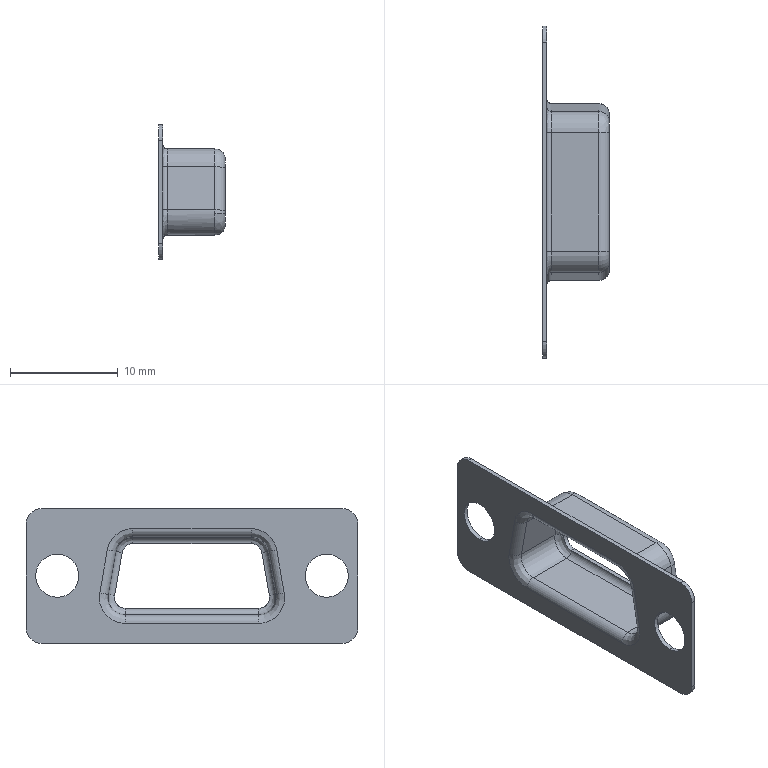Part | STEP file | SHELL | 1 solid | 72 faces | box 6.2 x 30.8 x 12.55 mm | volume 200.201 mm3 | cylinder 36 | plane 18 | spline 13 | other 4 | torus 1 | commonest cylinder face diameters 2 x8 4 x8 0.8 x4 1.2 x4 1.6 x4 3 x4